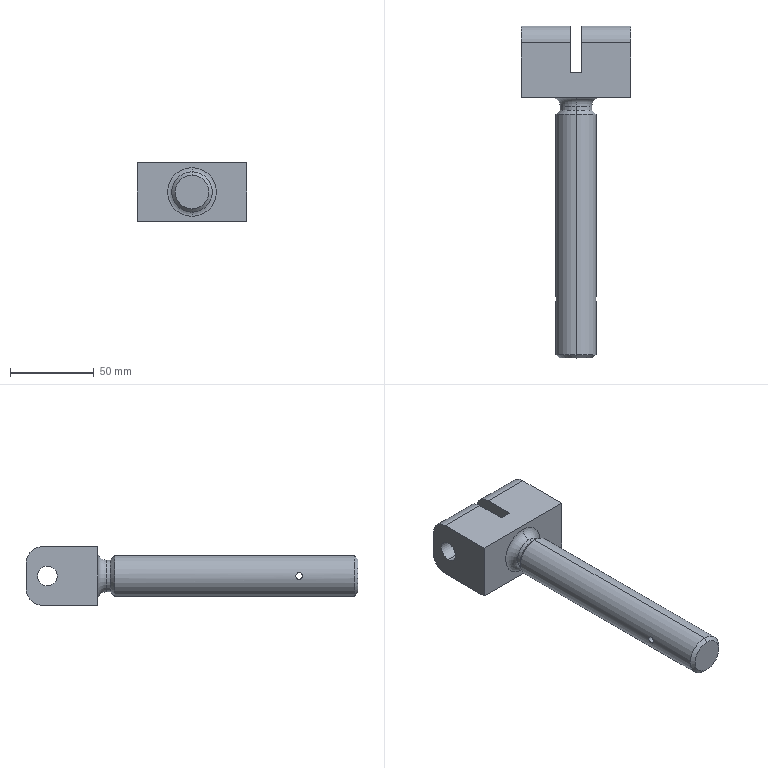Part | SolidWorks | features MBimport 1 | 1 solid | 31 faces | box 65.4 x 197.7 x 35 mm | volume 150563 mm3 | cylinder 14 | plane 11 | cone 4 | torus 2 | commonest cylinder face diameters 11.775 x4 20 x4 4 x2 19 x2 24 x2
STEP:
#1=CARTESIAN_POINT('',(20.868,-128.108,12.8));
#2=VERTEX_POINT('',#1);
#3=CARTESIAN_POINT('',(44.532,-128.108,12.8));
#4=VERTEX_POINT('',#3);
#5=CARTESIAN_POINT('',(0.,-128.108,12.8));
#6=DIRECTION('',(1.,0.,0.));
#7=VECTOR('',#6,1000.);
#8=LINE('',#5,#7);
#9=EDGE_CURVE('',#2,#4,#8,.T.);
#10=ORIENTED_EDGE('',*,*,#9,.F.);
#11=CARTESIAN_POINT('',(20.868,-128.108,8.8));
#12=VERTEX_POINT('',#11);
#13=CARTESIAN_POINT('',(20.868,-128.108,12.8));
#14=CARTESIAN_POINT('',(20.868,-127.984,12.8));
#15=CARTESIAN_POINT('',(20.866,-127.857,12.789));
#16=CARTESIAN_POINT('',(20.86,-127.664,12.751));
#17=CARTESIAN_POINT('',(20.857,-127.599,12.736));
#18=CARTESIAN_POINT('',(20.852,-127.503,12.707));
#19=CARTESIAN_POINT('',(20.85,-127.454,12.691));
#20=CARTESIAN_POINT('',(20.847,-127.398,12.67));
#21=CARTESIAN_POINT('',(20.845,-127.37,12.659));
#22=CARTESIAN_POINT('',(20.844,-127.358,12.654));
#23=CARTESIAN_POINT('',(20.844,-127.35,12.651));
#24=CARTESIAN_POINT('',(20.843,-127.345,12.649));
#25=CARTESIAN_POINT('',(20.838,-127.261,12.614));
#26=CARTESIAN_POINT('',(20.83,-127.162,12.567));
#27=CARTESIAN_POINT('',(20.81,-126.94,12.429));
#28=CARTESIAN_POINT('',(20.798,-126.816,12.337));
#29=CARTESIAN_POINT('',(20.769,-126.573,12.094));
#30=CARTESIAN_POINT('',(20.757,-126.482,11.972));
#31=CARTESIAN_POINT('',(20.742,-126.378,11.806));
#32=CARTESIAN_POINT('',(20.738,-126.349,11.753));
#33=CARTESIAN_POINT('',(20.732,-126.311,11.679));
#34=CARTESIAN_POINT('',(20.731,-126.3,11.656));
#35=CARTESIAN_POINT('',(20.728,-126.284,11.622));
#36=CARTESIAN_POINT('',(20.727,-126.277,11.605));
#37=CARTESIAN_POINT('',(20.726,-126.269,11.586));
#38=CARTESIAN_POINT('',(20.725,-126.265,11.578));
#39=CARTESIAN_POINT('',(20.725,-126.263,11.573));
#40=CARTESIAN_POINT('',(20.725,-126.263,11.572));
#41=CARTESIAN_POINT('',(20.708,-126.155,11.313));
#42=CARTESIAN_POINT('',(20.7,-126.108,11.049));
#43=CARTESIAN_POINT('',(20.7,-126.108,10.677));
#44=CARTESIAN_POINT('',(20.702,-126.119,10.55));
#45=CARTESIAN_POINT('',(20.708,-126.156,10.357));
#46=CARTESIAN_POINT('',(20.711,-126.172,10.292));
#47=CARTESIAN_POINT('',(20.715,-126.201,10.195));
#48=CARTESIAN_POINT('',(20.718,-126.217,10.147));
#49=CARTESIAN_POINT('',(20.721,-126.238,10.091));
#50=CARTESIAN_POINT('',(20.723,-126.249,10.063));
#51=CARTESIAN_POINT('',(20.723,-126.253,10.051));
#52=CARTESIAN_POINT('',(20.724,-126.257,10.043));
#53=CARTESIAN_POINT('',(20.724,-126.259,10.037));
#54=CARTESIAN_POINT('',(20.73,-126.294,9.952));
#55=CARTESIAN_POINT('',(20.737,-126.342,9.852));
#56=CARTESIAN_POINT('',(20.757,-126.481,9.63));
#57=CARTESIAN_POINT('',(20.769,-126.57,9.51));
#58=CARTESIAN_POINT('',(20.798,-126.815,9.264));
#59=CARTESIAN_POINT('',(20.81,-126.938,9.173));
#60=CARTESIAN_POINT('',(20.825,-127.104,9.069));
#61=CARTESIAN_POINT('',(20.83,-127.157,9.04));
#62=CARTESIAN_POINT('',(20.835,-127.23,9.003));
#63=CARTESIAN_POINT('',(20.837,-127.253,8.992));
#64=CARTESIAN_POINT('',(20.839,-127.287,8.976));
#65=CARTESIAN_POINT('',(20.841,-127.303,8.969));
#66=CARTESIAN_POINT('',(20.842,-127.322,8.961));
#67=CARTESIAN_POINT('',(20.842,-127.329,8.958));
#68=CARTESIAN_POINT('',(20.843,-127.335,8.956));
#69=CARTESIAN_POINT('',(20.843,-127.336,8.955));
#70=CARTESIAN_POINT('',(20.86,-127.596,8.847));
#71=CARTESIAN_POINT('',(20.868,-127.86,8.8));
#72=CARTESIAN_POINT('',(20.868,-128.108,8.8));
#73=B_SPLINE_CURVE_WITH_KNOTS('',3,(#13,#14,#15,#16,#17,#18,#19,#20,#21,#22,#23,#24,#25,#26,#27,#28,#29,#30,#31,#32,#33,#34,#35,#36,#37,#38,#39,#40,#41,#42,#43,#44,#45,#46,#47,#48,#49,#50,#51,#52,#53,#54,#55,#56,#57,#58,#59,#60,#61,#62,#63,#64,#65,#66,#67,#68,#69,#70,#71,#72),.UNSPECIFIED.,.F.,.F.,(4,2,2,1,1,1,2,2,2,2,2,2,2,1,1,2,2,2,2,2,1,1,1,2,2,2,2,2,2,2,1,1,2,2,4),(0.,0.0625,0.09375,0.1094,0.1172,0.1211,0.123,0.125,0.1875,0.25,0.3125,0.3438,0.3594,0.3672,0.3711,0.373,0.375,0.5,0.5625,0.5938,0.6094,0.6172,0.6211,0.623,0.625,0.6875,0.75,0.8125,0.8438,0.8594,0.8672,0.8711,0.873,0.875,1.),.UNSPECIFIED.);
#74=EDGE_CURVE('',#2,#12,#73,.T.);
#75=ORIENTED_EDGE('',*,*,#74,.T.);
#76=CARTESIAN_POINT('',(44.532,-128.108,8.8));
#77=VERTEX_POINT('',#76);
#78=CARTESIAN_POINT('',(0.,-128.108,8.8));
#79=DIRECTION('',(1.,0.,0.));
#80=VECTOR('',#79,1000.);
#81=LINE('',#78,#80);
#82=EDGE_CURVE('',#12,#77,#81,.T.);
#83=ORIENTED_EDGE('',*,*,#82,.T.);
#84=CARTESIAN_POINT('',(44.532,-128.108,8.8));
#85=CARTESIAN_POINT('',(44.532,-127.984,8.8));
#86=CARTESIAN_POINT('',(44.534,-127.856,8.812));
#87=CARTESIAN_POINT('',(44.54,-127.663,8.849));
#88=CARTESIAN_POINT('',(44.543,-127.599,8.865));
#89=CARTESIAN_POINT('',(44.548,-127.502,8.894));
#90=CARTESIAN_POINT('',(44.55,-127.453,8.91));
#91=CARTESIAN_POINT('',(44.553,-127.397,8.93));
#92=CARTESIAN_POINT('',(44.555,-127.369,8.941));
#93=CARTESIAN_POINT('',(44.556,-127.357,8.946));
#94=CARTESIAN_POINT('',(44.556,-127.349,8.95));
#95=CARTESIAN_POINT('',(44.557,-127.344,8.952));
#96=CARTESIAN_POINT('',(44.562,-127.26,8.987));
#97=CARTESIAN_POINT('',(44.57,-127.161,9.034));
#98=CARTESIAN_POINT('',(44.585,-126.994,9.137));
#99=CARTESIAN_POINT('',(44.59,-126.936,9.178));
#100=CARTESIAN_POINT('',(44.602,-126.816,9.271));
#101=CARTESIAN_POINT('',(44.609,-126.754,9.326));
#102=CARTESIAN_POINT('',(44.631,-126.572,9.507));
#103=CARTESIAN_POINT('',(44.643,-126.481,9.629));
#104=CARTESIAN_POINT('',(44.658,-126.377,9.795));
#105=CARTESIAN_POINT('',(44.662,-126.348,9.848));
#106=CARTESIAN_POINT('',(44.668,-126.311,9.922));
#107=CARTESIAN_POINT('',(44.669,-126.299,9.946));
#108=CARTESIAN_POINT('',(44.672,-126.284,9.98));
#109=CARTESIAN_POINT('',(44.673,-126.276,9.997));
#110=CARTESIAN_POINT('',(44.674,-126.268,10.015));
#111=CARTESIAN_POINT('',(44.675,-126.265,10.023));
#112=CARTESIAN_POINT('',(44.675,-126.263,10.029));
#113=CARTESIAN_POINT('',(44.675,-126.262,10.03));
#114=CARTESIAN_POINT('',(44.692,-126.155,10.289));
#115=CARTESIAN_POINT('',(44.7,-126.108,10.551));
#116=CARTESIAN_POINT('',(44.7,-126.108,10.923));
#117=CARTESIAN_POINT('',(44.698,-126.119,11.051));
#118=CARTESIAN_POINT('',(44.692,-126.156,11.244));
#119=CARTESIAN_POINT('',(44.689,-126.172,11.308));
#120=CARTESIAN_POINT('',(44.685,-126.201,11.405));
#121=CARTESIAN_POINT('',(44.682,-126.217,11.453));
#122=CARTESIAN_POINT('',(44.679,-126.238,11.51));
#123=CARTESIAN_POINT('',(44.677,-126.249,11.538));
#124=CARTESIAN_POINT('',(44.677,-126.253,11.55));
#125=CARTESIAN_POINT('',(44.676,-126.257,11.558));
#126=CARTESIAN_POINT('',(44.676,-126.259,11.563));
#127=CARTESIAN_POINT('',(44.67,-126.294,11.649));
#128=CARTESIAN_POINT('',(44.663,-126.342,11.749));
#129=CARTESIAN_POINT('',(44.643,-126.481,11.971));
#130=CARTESIAN_POINT('',(44.631,-126.571,12.092));
#131=CARTESIAN_POINT('',(44.602,-126.816,12.337));
#132=CARTESIAN_POINT('',(44.59,-126.939,12.428));
#133=CARTESIAN_POINT('',(44.575,-127.106,12.532));
#134=CARTESIAN_POINT('',(44.57,-127.158,12.561));
#135=CARTESIAN_POINT('',(44.565,-127.232,12.598));
#136=CARTESIAN_POINT('',(44.563,-127.255,12.609));
#137=CARTESIAN_POINT('',(44.56,-127.289,12.625));
#138=CARTESIAN_POINT('',(44.559,-127.305,12.632));
#139=CARTESIAN_POINT('',(44.558,-127.324,12.64));
#140=CARTESIAN_POINT('',(44.558,-127.332,12.643));
#141=CARTESIAN_POINT('',(44.557,-127.337,12.646));
#142=CARTESIAN_POINT('',(44.557,-127.338,12.646));
#143=CARTESIAN_POINT('',(44.54,-127.597,12.754));
#144=CARTESIAN_POINT('',(44.532,-127.86,12.8));
#145=CARTESIAN_POINT('',(44.532,-128.108,12.8));
#146=B_SPLINE_CURVE_WITH_KNOTS('',3,(#84,#85,#86,#87,#88,#89,#90,#91,#92,#93,#94,#95,#96,#97,#98,#99,#100,#101,#102,#103,#104,#105,#106,#107,#108,#109,#110,#111,#112,#113,#114,#115,#116,#117,#118,#119,#120,#121,#122,#123,#124,#125,#126,#127,#128,#129,#130,#131,#132,#133,#134,#135,#136,#137,#138,#139,#140,#141,#142,#143,#144,#145),.UNSPECIFIED.,.F.,.F.,(4,2,2,1,1,1,2,2,2,2,2,2,2,2,1,1,2,2,2,2,2,1,1,1,2,2,2,2,2,2,2,1,1,2,2,4),(0.,0.0625,0.09375,0.1094,0.1172,0.1211,0.123,0.125,0.1875,0.2188,0.25,0.3125,0.3438,0.3594,0.3672,0.3711,0.373,0.375,0.5,0.5625,0.5938,0.6094,0.6172,0.6211,0.623,0.625,0.6875,0.75,0.8125,0.8437,0.8594,0.8672,0.8711,0.873,0.875,1.),.UNSPECIFIED.);
#147=EDGE_CURVE('',#77,#4,#146,.T.);
#148=ORIENTED_EDGE('',*,*,#147,.T.);
#149=EDGE_LOOP('',(#10,#75,#83,#148));
#150=FACE_OUTER_BOUND('',#149,.T.);
#151=CARTESIAN_POINT('',(0.,-128.108,10.8));
#152=DIRECTION('',(1.,0.,0.));
#153=DIRECTION('',(0.,0.,-1.));
#154=AXIS2_PLACEMENT_3D('',#151,#152,#153);
#155=CYLINDRICAL_SURFACE('',#154,2.);
#156=ADVANCED_FACE('',(#150),#155,.F.);
#157=CARTESIAN_POINT('',(36.2,21.892,16.688));
#158=VERTEX_POINT('',#157);
#159=CARTESIAN_POINT('',(36.2,21.892,4.912));
#160=VERTEX_POINT('',#159);
#161=CARTESIAN_POINT('',(36.2,21.892,10.8));
#162=DIRECTION('',(-1.,0.,0.));
#163=DIRECTION('',(0.,0.,1.));
#164=AXIS2_PLACEMENT_3D('',#161,#162,#163);
#165=CIRCLE('',#164,5.888);
#166=EDGE_CURVE('',#158,#160,#165,.T.);
#167=ORIENTED_EDGE('',*,*,#166,.F.);
#168=CARTESIAN_POINT('',(36.2,21.892,10.8));
#169=DIRECTION('',(-1.,0.,0.));
#170=DIRECTION('',(0.,0.,1.));
#171=AXIS2_PLACEMENT_3D('',#168,#169,#170);
#172=CIRCLE('',#171,5.888);
#173=EDGE_CURVE('',#160,#158,#172,.T.);
#174=ORIENTED_EDGE('',*,*,#173,.F.);
#175=EDGE_LOOP('',(#167,#174));
#176=FACE_BOUND('',#175,.T.);
#177=CARTESIAN_POINT('',(36.2,34.592,3.3));
#178=VERTEX_POINT('',#177);
#179=CARTESIAN_POINT('',(36.2,24.592,-6.7));
#180=VERTEX_POINT('',#179);
#181=CARTESIAN_POINT('',(36.2,24.592,3.3));
#182=DIRECTION('',(-1.,0.,0.));
#183=DIRECTION('',(0.,0.,1.));
#184=AXIS2_PLACEMENT_3D('',#181,#182,#183);
#185=CIRCLE('',#184,10.);
#186=EDGE_CURVE('',#178,#180,#185,.T.);
#187=ORIENTED_EDGE('',*,*,#186,.T.);
#188=CARTESIAN_POINT('',(36.2,6.592,-6.7));
#189=VERTEX_POINT('',#188);
#190=CARTESIAN_POINT('',(36.2,24.592,-6.7));
#191=DIRECTION('',(0.,-1.,0.));
#192=VECTOR('',#191,1000.);
#193=LINE('',#190,#192);
#194=EDGE_CURVE('',#180,#189,#193,.T.);
#195=ORIENTED_EDGE('',*,*,#194,.T.);
#196=CARTESIAN_POINT('',(36.2,6.592,28.3));
#197=VERTEX_POINT('',#196);
#198=CARTESIAN_POINT('',(36.2,6.592,335.997));
#199=DIRECTION('',(0.,0.,-1.));
#200=VECTOR('',#199,1000.);
#201=LINE('',#198,#200);
#202=EDGE_CURVE('',#197,#189,#201,.T.);
#203=ORIENTED_EDGE('',*,*,#202,.F.);
#204=CARTESIAN_POINT('',(36.2,24.592,28.3));
#205=VERTEX_POINT('',#204);
#206=CARTESIAN_POINT('',(36.2,24.592,28.3));
#207=DIRECTION('',(0.,1.,0.));
#208=VECTOR('',#207,1000.);
#209=LINE('',#206,#208);
#210=EDGE_CURVE('',#197,#205,#209,.T.);
#211=ORIENTED_EDGE('',*,*,#210,.T.);
#212=CARTESIAN_POINT('',(36.2,34.592,18.3));
#213=VERTEX_POINT('',#212);
#214=CARTESIAN_POINT('',(36.2,24.592,18.3));
#215=DIRECTION('',(-1.,0.,0.));
#216=DIRECTION('',(0.,0.,1.));
#217=AXIS2_PLACEMENT_3D('',#214,#215,#216);
#218=CIRCLE('',#217,10.);
#219=EDGE_CURVE('',#205,#213,#218,.T.);
#220=ORIENTED_EDGE('',*,*,#219,.T.);
#221=CARTESIAN_POINT('',(36.2,34.592,335.997));
#222=DIRECTION('',(0.,0.,-1.));
#223=VECTOR('',#222,1000.);
#224=LINE('',#221,#223);
#225=EDGE_CURVE('',#213,#178,#224,.T.);
#226=ORIENTED_EDGE('',*,*,#225,.T.);
#227=EDGE_LOOP('',(#187,#195,#203,#211,#220,#226));
#228=FACE_OUTER_BOUND('',#227,.T.);
#229=CARTESIAN_POINT('',(36.2,6.592,335.997));
#230=DIRECTION('',(-1.,0.,0.));
#231=DIRECTION('',(0.,0.,1.));
#232=AXIS2_PLACEMENT_3D('',#229,#230,#231);
#233=PLANE('',#232);
#234=ADVANCED_FACE('',(#176,#228),#233,.T.);
#235=CARTESIAN_POINT('',(29.2,21.892,16.688));
#236=VERTEX_POINT('',#235);
#237=CARTESIAN_POINT('',(29.2,21.892,4.912));
#238=VERTEX_POINT('',#237);
#239=CARTESIAN_POINT('',(29.2,21.892,10.8));
#240=DIRECTION('',(1.,0.,0.));
#241=DIRECTION('',(0.,1.,0.));
#242=AXIS2_PLACEMENT_3D('',#239,#240,#241);
#243=CIRCLE('',#242,5.888);
#244=EDGE_CURVE('',#236,#238,#243,.T.);
#245=ORIENTED_EDGE('',*,*,#244,.F.);
#246=CARTESIAN_POINT('',(29.2,21.892,10.8));
#247=DIRECTION('',(1.,0.,0.));
#248=DIRECTION('',(0.,1.,0.));
#249=AXIS2_PLACEMENT_3D('',#246,#247,#248);
#250=CIRCLE('',#249,5.888);
#251=EDGE_CURVE('',#238,#236,#250,.T.);
#252=ORIENTED_EDGE('',*,*,#251,.F.);
#253=EDGE_LOOP('',(#245,#252));
#254=FACE_BOUND('',#253,.T.);
#255=CARTESIAN_POINT('',(29.2,6.592,28.3));
#256=VERTEX_POINT('',#255);
#257=CARTESIAN_POINT('',(29.2,6.592,-6.7));
#258=VERTEX_POINT('',#257);
#259=CARTESIAN_POINT('',(29.2,6.592,335.997));
#260=DIRECTION('',(0.,0.,-1.));
#261=VECTOR('',#260,1000.);
#262=LINE('',#259,#261);
#263=EDGE_CURVE('',#256,#258,#262,.T.);
#264=ORIENTED_EDGE('',*,*,#263,.T.);
#265=CARTESIAN_POINT('',(29.2,24.592,-6.7));
#266=VERTEX_POINT('',#265);
#267=CARTESIAN_POINT('',(29.2,24.592,-6.7));
#268=DIRECTION('',(0.,1.,0.));
#269=VECTOR('',#268,1000.);
#270=LINE('',#267,#269);
#271=EDGE_CURVE('',#258,#266,#270,.T.);
#272=ORIENTED_EDGE('',*,*,#271,.T.);
#273=CARTESIAN_POINT('',(29.2,34.592,3.3));
#274=VERTEX_POINT('',#273);
#275=CARTESIAN_POINT('',(29.2,24.592,3.3));
#276=DIRECTION('',(1.,0.,0.));
#277=DIRECTION('',(0.,1.,0.));
#278=AXIS2_PLACEMENT_3D('',#275,#276,#277);
#279=CIRCLE('',#278,10.);
#280=EDGE_CURVE('',#266,#274,#279,.T.);
#281=ORIENTED_EDGE('',*,*,#280,.T.);
#282=CARTESIAN_POINT('',(29.2,34.592,18.3));
#283=VERTEX_POINT('',#282);
#284=CARTESIAN_POINT('',(29.2,34.592,335.997));
#285=DIRECTION('',(0.,0.,-1.));
#286=VECTOR('',#285,1000.);
#287=LINE('',#284,#286);
#288=EDGE_CURVE('',#283,#274,#287,.T.);
#289=ORIENTED_EDGE('',*,*,#288,.F.);
#290=CARTESIAN_POINT('',(29.2,24.592,28.3));
#291=VERTEX_POINT('',#290);
#292=CARTESIAN_POINT('',(29.2,24.592,18.3));
#293=DIRECTION('',(1.,0.,0.));
#294=DIRECTION('',(0.,1.,0.));
#295=AXIS2_PLACEMENT_3D('',#292,#293,#294);
#296=CIRCLE('',#295,10.);
#297=EDGE_CURVE('',#283,#291,#296,.T.);
#298=ORIENTED_EDGE('',*,*,#297,.T.);
#299=CARTESIAN_POINT('',(29.2,24.592,28.3));
#300=DIRECTION('',(0.,-1.,0.));
#301=VECTOR('',#300,1000.);
#302=LINE('',#299,#301);
#303=EDGE_CURVE('',#291,#256,#302,.T.);
#304=ORIENTED_EDGE('',*,*,#303,.T.);
#305=EDGE_LOOP('',(#264,#272,#281,#289,#298,#304));
#306=FACE_OUTER_BOUND('',#305,.T.);
#307=CARTESIAN_POINT('',(29.2,34.592,335.997));
#308=DIRECTION('',(1.,0.,0.));
#309=DIRECTION('',(0.,1.,0.));
#310=AXIS2_PLACEMENT_3D('',#307,#308,#309);
#311=PLANE('',#310);
#312=ADVANCED_FACE('',(#254,#306),#311,.T.);
#313=ORIENTED_EDGE('',*,*,#202,.T.);
#314=CARTESIAN_POINT('',(65.4,6.592,-6.7));
#315=DIRECTION('',(-1.,0.,0.));
#316=VECTOR('',#315,1000.);
#317=LINE('',#314,#316);
#318=EDGE_CURVE('',#189,#258,#317,.T.);
#319=ORIENTED_EDGE('',*,*,#318,.T.);
#320=ORIENTED_EDGE('',*,*,#263,.F.);
#321=CARTESIAN_POINT('',(65.4,6.592,28.3));
#322=DIRECTION('',(1.,0.,0.));
#323=VECTOR('',#322,1000.);
#324=LINE('',#321,#323);
#325=EDGE_CURVE('',#256,#197,#324,.T.);
#326=ORIENTED_EDGE('',*,*,#325,.T.);
#327=EDGE_LOOP('',(#313,#319,#320,#326));
#328=FACE_OUTER_BOUND('',#327,.T.);
#329=CARTESIAN_POINT('',(29.2,6.592,335.997));
#330=DIRECTION('',(0.,1.,0.));
#331=DIRECTION('',(1.,0.,0.));
#332=AXIS2_PLACEMENT_3D('',#329,#330,#331);
#333=PLANE('',#332);
#334=ADVANCED_FACE('',(#328),#333,.T.);
#335=CARTESIAN_POINT('',(32.7,-163.108,0.8001));
#336=VERTEX_POINT('',#335);
#337=CARTESIAN_POINT('',(32.7,-161.108,-1.2));
#338=VERTEX_POINT('',#337);
#339=CARTESIAN_POINT('',(32.7,-161.108,-1.2));
#340=DIRECTION('',(0.,0.7071,-0.7071));
#341=VECTOR('',#340,1000.);
#342=LINE('',#339,#341);
#343=EDGE_CURVE('',#336,#338,#342,.T.);
#344=ORIENTED_EDGE('',*,*,#343,.F.);
#345=CARTESIAN_POINT('',(32.7,-163.108,20.8));
#346=VERTEX_POINT('',#345);
#347=CARTESIAN_POINT('',(32.7,-163.108,10.8));
#348=DIRECTION('',(0.,-1.,0.));
#349=DIRECTION('',(0.,0.,-1.));
#350=AXIS2_PLACEMENT_3D('',#347,#348,#349);
#351=CIRCLE('',#350,10.);
#352=EDGE_CURVE('',#346,#336,#351,.T.);
#353=ORIENTED_EDGE('',*,*,#352,.F.);
#354=CARTESIAN_POINT('',(32.7,-161.108,22.8));
#355=VERTEX_POINT('',#354);
#356=CARTESIAN_POINT('',(32.7,-161.108,22.8));
#357=DIRECTION('',(0.,0.7071,0.7071));
#358=VECTOR('',#357,1000.);
#359=LINE('',#356,#358);
#360=EDGE_CURVE('',#346,#355,#359,.T.);
#361=ORIENTED_EDGE('',*,*,#360,.T.);
#362=CARTESIAN_POINT('',(32.7,-161.108,10.8));
#363=DIRECTION('',(0.,1.,0.));
#364=DIRECTION('',(0.,0.,-1.));
#365=AXIS2_PLACEMENT_3D('',#362,#363,#364);
#366=CIRCLE('',#365,12.);
#367=EDGE_CURVE('',#338,#355,#366,.T.);
#368=ORIENTED_EDGE('',*,*,#367,.F.);
#369=EDGE_LOOP('',(#344,#353,#361,#368));
#370=FACE_OUTER_BOUND('',#369,.T.);
#371=CARTESIAN_POINT('',(32.7,-161.108,10.8));
#372=DIRECTION('',(0.,1.,0.));
#373=DIRECTION('',(0.,0.,1.));
#374=AXIS2_PLACEMENT_3D('',#371,#372,#373);
#375=CONICAL_SURFACE('',#374,12.,0.7854);
#376=ADVANCED_FACE('',(#370),#375,.T.);
#377=ORIENTED_EDGE('',*,*,#352,.T.);
#378=CARTESIAN_POINT('',(32.7,-163.108,10.8));
#379=DIRECTION('',(0.,-1.,0.));
#380=DIRECTION('',(0.,0.,-1.));
#381=AXIS2_PLACEMENT_3D('',#378,#379,#380);
#382=CIRCLE('',#381,10.);
#383=EDGE_CURVE('',#336,#346,#382,.T.);
#384=ORIENTED_EDGE('',*,*,#383,.T.);
#385=EDGE_LOOP('',(#377,#384));
#386=FACE_OUTER_BOUND('',#385,.T.);
#387=CARTESIAN_POINT('',(32.7,-163.108,0.));
#388=DIRECTION('',(0.,-1.,0.));
#389=DIRECTION('',(0.,0.,-1.));
#390=AXIS2_PLACEMENT_3D('',#387,#388,#389);
#391=PLANE('',#390);
#392=ADVANCED_FACE('',(#386),#391,.T.);
#393=CARTESIAN_POINT('',(20.868,-128.108,8.8));
#394=CARTESIAN_POINT('',(20.868,-128.232,8.8));
#395=CARTESIAN_POINT('',(20.866,-128.359,8.812));
#396=CARTESIAN_POINT('',(20.86,-128.552,8.849));
#397=CARTESIAN_POINT('',(20.857,-128.617,8.865));
#398=CARTESIAN_POINT('',(20.852,-128.714,8.894));
#399=CARTESIAN_POINT('',(20.85,-128.762,8.91));
#400=CARTESIAN_POINT('',(20.847,-128.818,8.93));
#401=CARTESIAN_POINT('',(20.845,-128.846,8.941));
#402=CARTESIAN_POINT('',(20.844,-128.858,8.946));
#403=CARTESIAN_POINT('',(20.844,-128.866,8.95));
#404=CARTESIAN_POINT('',(20.843,-128.872,8.952));
#405=CARTESIAN_POINT('',(20.838,-128.956,8.987));
#406=CARTESIAN_POINT('',(20.83,-129.055,9.034));
#407=CARTESIAN_POINT('',(20.815,-129.221,9.137));
#408=CARTESIAN_POINT('',(20.81,-129.28,9.178));
#409=CARTESIAN_POINT('',(20.798,-129.399,9.271));
#410=CARTESIAN_POINT('',(20.791,-129.462,9.326));
#411=CARTESIAN_POINT('',(20.769,-129.643,9.507));
#412=CARTESIAN_POINT('',(20.757,-129.734,9.629));
#413=CARTESIAN_POINT('',(20.742,-129.838,9.795));
#414=CARTESIAN_POINT('',(20.738,-129.868,9.848));
#415=CARTESIAN_POINT('',(20.732,-129.905,9.922));
#416=CARTESIAN_POINT('',(20.731,-129.916,9.946));
#417=CARTESIAN_POINT('',(20.728,-129.932,9.98));
#418=CARTESIAN_POINT('',(20.727,-129.939,9.997));
#419=CARTESIAN_POINT('',(20.726,-129.947,10.015));
#420=CARTESIAN_POINT('',(20.725,-129.951,10.023));
#421=CARTESIAN_POINT('',(20.725,-129.953,10.029));
#422=CARTESIAN_POINT('',(20.725,-129.953,10.03));
#423=CARTESIAN_POINT('',(20.708,-130.061,10.289));
#424=CARTESIAN_POINT('',(20.7,-130.108,10.551));
#425=CARTESIAN_POINT('',(20.7,-130.108,10.923));
#426=CARTESIAN_POINT('',(20.702,-130.096,11.051));
#427=CARTESIAN_POINT('',(20.708,-130.059,11.244));
#428=CARTESIAN_POINT('',(20.711,-130.043,11.308));
#429=CARTESIAN_POINT('',(20.715,-130.014,11.405));
#430=CARTESIAN_POINT('',(20.718,-129.999,11.453));
#431=CARTESIAN_POINT('',(20.721,-129.978,11.51));
#432=CARTESIAN_POINT('',(20.723,-129.967,11.538));
#433=CARTESIAN_POINT('',(20.723,-129.962,11.55));
#434=CARTESIAN_POINT('',(20.724,-129.959,11.558));
#435=CARTESIAN_POINT('',(20.724,-129.957,11.563));
#436=CARTESIAN_POINT('',(20.73,-129.921,11.649));
#437=CARTESIAN_POINT('',(20.737,-129.873,11.749));
#438=CARTESIAN_POINT('',(20.757,-129.735,11.971));
#439=CARTESIAN_POINT('',(20.769,-129.645,12.092));
#440=CARTESIAN_POINT('',(20.798,-129.399,12.337));
#441=CARTESIAN_POINT('',(20.81,-129.276,12.428));
#442=CARTESIAN_POINT('',(20.825,-129.11,12.532));
#443=CARTESIAN_POINT('',(20.83,-129.057,12.561));
#444=CARTESIAN_POINT('',(20.835,-128.984,12.598));
#445=CARTESIAN_POINT('',(20.837,-128.96,12.609));
#446=CARTESIAN_POINT('',(20.84,-128.927,12.625));
#447=CARTESIAN_POINT('',(20.841,-128.91,12.632));
#448=CARTESIAN_POINT('',(20.842,-128.892,12.64));
#449=CARTESIAN_POINT('',(20.842,-128.884,12.643));
#450=CARTESIAN_POINT('',(20.843,-128.879,12.646));
#451=CARTESIAN_POINT('',(20.843,-128.878,12.646));
#452=CARTESIAN_POINT('',(20.86,-128.618,12.754));
#453=CARTESIAN_POINT('',(20.868,-128.355,12.8));
#454=CARTESIAN_POINT('',(20.868,-128.108,12.8));
#455=B_SPLINE_CURVE_WITH_KNOTS('',3,(#393,#394,#395,#396,#397,#398,#399,#400,#401,#402,#403,#404,#405,#406,#407,#408,#409,#410,#411,#412,#413,#414,#415,#416,#417,#418,#419,#420,#421,#422,#423,#424,#425,#426,#427,#428,#429,#430,#431,#432,#433,#434,#435,#436,#437,#438,#439,#440,#441,#442,#443,#444,#445,#446,#447,#448,#449,#450,#451,#452,#453,#454),.UNSPECIFIED.,.F.,.F.,(4,2,2,1,1,1,2,2,2,2,2,2,2,2,1,1,2,2,2,2,2,1,1,1,2,2,2,2,2,2,2,1,1,2,2,4),(0.,0.0625,0.09375,0.1094,0.1172,0.1211,0.123,0.125,0.1875,0.2187,0.25,0.3125,0.3437,0.3594,0.3672,0.3711,0.373,0.375,0.5,0.5625,0.5937,0.6094,0.6172,0.6211,0.623,0.625,0.6875,0.75,0.8125,0.8437,0.8594,0.8672,0.8711,0.873,0.875,1.),.UNSPECIFIED.);
#456=EDGE_CURVE('',#12,#2,#455,.T.);
#457=ORIENTED_EDGE('',*,*,#456,.F.);
#458=ORIENTED_EDGE('',*,*,#74,.F.);
#459=EDGE_LOOP('',(#457,#458));
#460=FACE_BOUND('',#459,.T.);
#461=CARTESIAN_POINT('',(32.7,-18.108,-1.2));
#462=VERTEX_POINT('',#461);
#463=CARTESIAN_POINT('',(32.7,34.592,-1.2));
#464=DIRECTION('',(0.,1.,0.));
#465=VECTOR('',#464,1000.);
#466=LINE('',#463,#465);
#467=EDGE_CURVE('',#338,#462,#466,.T.);
#468=ORIENTED_EDGE('',*,*,#467,.F.);
#469=ORIENTED_EDGE('',*,*,#367,.T.);
#470=CARTESIAN_POINT('',(32.7,-18.108,22.8));
#471=VERTEX_POINT('',#470);
#472=CARTESIAN_POINT('',(32.7,34.592,22.8));
#473=DIRECTION('',(0.,1.,0.));
#474=VECTOR('',#473,1000.);
#475=LINE('',#472,#474);
#476=EDGE_CURVE('',#355,#471,#475,.T.);
#477=ORIENTED_EDGE('',*,*,#476,.T.);
#478=CARTESIAN_POINT('',(32.7,-18.108,10.8));
#479=DIRECTION('',(0.,1.,0.));
#480=DIRECTION('',(0.,0.,1.));
#481=AXIS2_PLACEMENT_3D('',#478,#479,#480);
#482=CIRCLE('',#481,12.);
#483=EDGE_CURVE('',#462,#471,#482,.T.);
#484=ORIENTED_EDGE('',*,*,#483,.F.);
#485=EDGE_LOOP('',(#468,#469,#477,#484));
#486=FACE_OUTER_BOUND('',#485,.T.);
#487=CARTESIAN_POINT('',(32.7,34.592,10.8));
#488=DIRECTION('',(0.,1.,0.));
#489=DIRECTION('',(0.,0.,1.));
#490=AXIS2_PLACEMENT_3D('',#487,#488,#489);
#491=CYLINDRICAL_SURFACE('',#490,12.);
#492=ADVANCED_FACE('',(#460,#486),#491,.T.);
#493=CARTESIAN_POINT('',(32.7,-15.608,20.3));
#494=VERTEX_POINT('',#493);
#495=CARTESIAN_POINT('',(32.7,-18.108,22.8));
#496=DIRECTION('',(0.,-0.7071,0.7071));
#497=VECTOR('',#496,1000.);
#498=LINE('',#495,#497);
#499=EDGE_CURVE('',#494,#471,#498,.T.);
#500=ORIENTED_EDGE('',*,*,#499,.F.);
#501=CARTESIAN_POINT('',(32.7,-15.608,1.3));
#502=VERTEX_POINT('',#501);
#503=CARTESIAN_POINT('',(32.7,-15.608,10.8));
#504=DIRECTION('',(0.,1.,0.));
#505=DIRECTION('',(0.,0.,1.));
#506=AXIS2_PLACEMENT_3D('',#503,#504,#505);
#507=CIRCLE('',#506,9.5);
#508=EDGE_CURVE('',#502,#494,#507,.T.);
#509=ORIENTED_EDGE('',*,*,#508,.F.);
#510=CARTESIAN_POINT('',(32.7,-18.108,-1.2));
#511=DIRECTION('',(0.,-0.7071,-0.7071));
#512=VECTOR('',#511,1000.);
#513=LINE('',#510,#512);
#514=EDGE_CURVE('',#502,#462,#513,.T.);
#515=ORIENTED_EDGE('',*,*,#514,.T.);
#516=ORIENTED_EDGE('',*,*,#483,.T.);
#517=EDGE_LOOP('',(#500,#509,#515,#516));
#518=FACE_OUTER_BOUND('',#517,.T.);
#519=CARTESIAN_POINT('',(32.7,-18.108,10.8));
#520=DIRECTION('',(0.,-1.,0.));
#521=DIRECTION('',(0.,0.,-1.));
#522=AXIS2_PLACEMENT_3D('',#519,#520,#521);
#523=CONICAL_SURFACE('',#522,12.,0.7854);
#524=ADVANCED_FACE('',(#518),#523,.T.);
#525=CARTESIAN_POINT('',(32.7,-13.108,1.3));
#526=VERTEX_POINT('',#525);
#527=CARTESIAN_POINT('',(32.7,34.592,1.3));
#528=DIRECTION('',(0.,1.,0.));
#529=VECTOR('',#528,1000.);
#530=LINE('',#527,#529);
#531=EDGE_CURVE('',#502,#526,#530,.T.);
#532=ORIENTED_EDGE('',*,*,#531,.F.);
#533=ORIENTED_EDGE('',*,*,#508,.T.);
#534=CARTESIAN_POINT('',(32.7,-13.108,20.3));
#535=VERTEX_POINT('',#534);
#536=CARTESIAN_POINT('',(32.7,34.592,20.3));
#537=DIRECTION('',(0.,1.,0.));
#538=VECTOR('',#537,1000.);
#539=LINE('',#536,#538);
#540=EDGE_CURVE('',#494,#535,#539,.T.);
#541=ORIENTED_EDGE('',*,*,#540,.T.);
#542=CARTESIAN_POINT('',(32.7,-13.108,10.8));
#543=DIRECTION('',(0.,1.,0.));
#544=DIRECTION('',(0.,0.,1.));
#545=AXIS2_PLACEMENT_3D('',#542,#543,#544);
#546=CIRCLE('',#545,9.5);
#547=EDGE_CURVE('',#526,#535,#546,.T.);
#548=ORIENTED_EDGE('',*,*,#547,.F.);
#549=EDGE_LOOP('',(#532,#533,#541,#548));
#550=FACE_OUTER_BOUND('',#549,.T.);
#551=CARTESIAN_POINT('',(32.7,34.592,10.8));
#552=DIRECTION('',(0.,1.,0.));
#553=DIRECTION('',(0.,0.,1.));
#554=AXIS2_PLACEMENT_3D('',#551,#552,#553);
#555=CYLINDRICAL_SURFACE('',#554,9.5);
#556=ADVANCED_FACE('',(#550),#555,.T.);
#557=CARTESIAN_POINT('',(32.7,-8.108,-3.7));
#558=VERTEX_POINT('',#557);
#559=CARTESIAN_POINT('',(32.7,-13.108,-3.7));
#560=DIRECTION('',(1.,0.,0.));
#561=DIRECTION('',(0.,0.,-1.));
#562=AXIS2_PLACEMENT_3D('',#559,#560,#561);
#563=CIRCLE('',#562,5.);
#564=EDGE_CURVE('',#558,#526,#563,.T.);
#565=ORIENTED_EDGE('',*,*,#564,.F.);
#566=CARTESIAN_POINT('',(32.7,-8.108,25.3));
#567=VERTEX_POINT('',#566);
#568=CARTESIAN_POINT('',(32.7,-8.108,10.8));
#569=DIRECTION('',(0.,1.,0.));
#570=DIRECTION('',(0.,0.,1.));
#571=AXIS2_PLACEMENT_3D('',#568,#569,#570);
#572=CIRCLE('',#571,14.5);
#573=EDGE_CURVE('',#567,#558,#572,.T.);
#574=ORIENTED_EDGE('',*,*,#573,.F.);
#575=CARTESIAN_POINT('',(32.7,-13.108,25.3));
#576=DIRECTION('',(-1.,0.,0.));
#577=DIRECTION('',(0.,0.,1.));
#578=AXIS2_PLACEMENT_3D('',#575,#576,#577);
#579=CIRCLE('',#578,5.);
#580=EDGE_CURVE('',#567,#535,#579,.T.);
#581=ORIENTED_EDGE('',*,*,#580,.T.);
#582=CARTESIAN_POINT('',(32.7,-13.108,10.8));
#583=DIRECTION('',(0.,1.,0.));
#584=DIRECTION('',(0.,0.,1.));
#585=AXIS2_PLACEMENT_3D('',#582,#583,#584);
#586=CIRCLE('',#585,9.5);
#587=EDGE_CURVE('',#535,#526,#586,.T.);
#588=ORIENTED_EDGE('',*,*,#587,.T.);
#589=EDGE_LOOP('',(#565,#574,#581,#588));
#590=FACE_OUTER_BOUND('',#589,.T.);
#591=CARTESIAN_POINT('',(32.7,-13.108,10.8));
#592=DIRECTION('',(0.,1.,0.));
#593=DIRECTION('',(0.,0.,1.));
#594=AXIS2_PLACEMENT_3D('',#591,#592,#593);
#595=TOROIDAL_SURFACE('',#594,14.5,5.);
#596=ADVANCED_FACE('',(#590),#595,.F.);
#597=ORIENTED_EDGE('',*,*,#573,.T.);
#598=CARTESIAN_POINT('',(32.7,-8.108,10.8));
#599=DIRECTION('',(0.,1.,0.));
#600=DIRECTION('',(0.,0.,1.));
#601=AXIS2_PLACEMENT_3D('',#598,#599,#600);
#602=CIRCLE('',#601,14.5);
#603=EDGE_CURVE('',#558,#567,#602,.T.);
#604=ORIENTED_EDGE('',*,*,#603,.T.);
#605=EDGE_LOOP('',(#597,#604));
#606=FACE_BOUND('',#605,.T.);
#607=CARTESIAN_POINT('',(0.,-8.108,28.3));
#608=VERTEX_POINT('',#607);
#609=CARTESIAN_POINT('',(0.,-8.108,-6.7));
#610=VERTEX_POINT('',#609);
#611=CARTESIAN_POINT('',(0.,-8.108,28.3));
#612=DIRECTION('',(0.,0.,-1.));
#613=VECTOR('',#612,1000.);
#614=LINE('',#611,#613);
#615=EDGE_CURVE('',#608,#610,#614,.T.);
#616=ORIENTED_EDGE('',*,*,#615,.T.);
#617=CARTESIAN_POINT('',(65.4,-8.108,-6.7));
#618=VERTEX_POINT('',#617);
#619=CARTESIAN_POINT('',(65.4,-8.108,-6.7));
#620=DIRECTION('',(-1.,0.,0.));
#621=VECTOR('',#620,1000.);
#622=LINE('',#619,#621);
#623=EDGE_CURVE('',#618,#610,#622,.T.);
#624=ORIENTED_EDGE('',*,*,#623,.F.);
#625=CARTESIAN_POINT('',(65.4,-8.108,28.3));
#626=VERTEX_POINT('',#625);
#627=CARTESIAN_POINT('',(65.4,-8.108,28.3));
#628=DIRECTION('',(0.,0.,-1.));
#629=VECTOR('',#628,1000.);
#630=LINE('',#627,#629);
#631=EDGE_CURVE('',#626,#618,#630,.T.);
#632=ORIENTED_EDGE('',*,*,#631,.F.);
#633=CARTESIAN_POINT('',(65.4,-8.108,28.3));
#634=DIRECTION('',(-1.,0.,0.));
#635=VECTOR('',#634,1000.);
#636=LINE('',#633,#635);
#637=EDGE_CURVE('',#626,#608,#636,.T.);
#638=ORIENTED_EDGE('',*,*,#637,.T.);
#639=EDGE_LOOP('',(#616,#624,#632,#638));
#640=FACE_OUTER_BOUND('',#639,.T.);
#641=CARTESIAN_POINT('',(65.4,-8.108,28.3));
#642=DIRECTION('',(0.,1.,0.));
#643=DIRECTION('',(1.,0.,0.));
#644=AXIS2_PLACEMENT_3D('',#641,#642,#643);
#645=PLANE('',#644);
#646=ADVANCED_FACE('',(#606,#640),#645,.F.);
#647=CARTESIAN_POINT('',(0.,34.592,18.3));
#648=VERTEX_POINT('',#647);
#649=CARTESIAN_POINT('',(65.4,34.592,18.3));
#650=DIRECTION('',(-1.,0.,0.));
#651=VECTOR('',#650,1000.);
#652=LINE('',#649,#651);
#653=EDGE_CURVE('',#283,#648,#652,.T.);
#654=ORIENTED_EDGE('',*,*,#653,.F.);
#655=ORIENTED_EDGE('',*,*,#288,.T.);
#656=CARTESIAN_POINT('',(0.,34.592,3.3));
#657=VERTEX_POINT('',#656);
#658=CARTESIAN_POINT('',(65.4,34.592,3.3));
#659=DIRECTION('',(-1.,0.,0.));
#660=VECTOR('',#659,1000.);
#661=LINE('',#658,#660);
#662=EDGE_CURVE('',#274,#657,#661,.T.);
#663=ORIENTED_EDGE('',*,*,#662,.T.);
#664=CARTESIAN_POINT('',(0.,34.592,18.3));
#665=DIRECTION('',(0.,0.,1.));
#666=VECTOR('',#665,1000.);
#667=LINE('',#664,#666);
#668=EDGE_CURVE('',#657,#648,#667,.T.);
#669=ORIENTED_EDGE('',*,*,#668,.T.);
#670=EDGE_LOOP('',(#654,#655,#663,#669));
#671=FACE_OUTER_BOUND('',#670,.T.);
#672=CARTESIAN_POINT('',(65.4,34.592,18.3));
#673=DIRECTION('',(0.,-1.,0.));
#674=DIRECTION('',(0.,0.,-1.));
#675=AXIS2_PLACEMENT_3D('',#672,#673,#674);
#676=PLANE('',#675);
#677=ADVANCED_FACE('',(#671),#676,.F.);
#678=CARTESIAN_POINT('',(0.,21.892,16.688));
#679=VERTEX_POINT('',#678);
#680=CARTESIAN_POINT('',(0.,21.892,4.912));
#681=VERTEX_POINT('',#680);
#682=CARTESIAN_POINT('',(0.,21.892,10.8));
#683=DIRECTION('',(1.,0.,0.));
#684=DIRECTION('',(0.,0.,-1.));
#685=AXIS2_PLACEMENT_3D('',#682,#683,#684);
#686=CIRCLE('',#685,5.888);
#687=EDGE_CURVE('',#679,#681,#686,.T.);
#688=ORIENTED_EDGE('',*,*,#687,.T.);
#689=CARTESIAN_POINT('',(0.,21.892,10.8));
#690=DIRECTION('',(1.,0.,0.));
#691=DIRECTION('',(0.,0.,-1.));
#692=AXIS2_PLACEMENT_3D('',#689,#690,#691);
#693=CIRCLE('',#692,5.888);
#694=EDGE_CURVE('',#681,#679,#693,.T.);
#695=ORIENTED_EDGE('',*,*,#694,.T.);
#696=EDGE_LOOP('',(#688,#695));
#697=FACE_BOUND('',#696,.T.);
#698=CARTESIAN_POINT('',(0.,24.592,-6.7));
#699=VERTEX_POINT('',#698);
#700=CARTESIAN_POINT('',(0.,24.592,-6.7));
#701=DIRECTION('',(0.,1.,0.));
#702=VECTOR('',#701,1000.);
#703=LINE('',#700,#702);
#704=EDGE_CURVE('',#610,#699,#703,.T.);
#705=ORIENTED_EDGE('',*,*,#704,.F.);
#706=ORIENTED_EDGE('',*,*,#615,.F.);
#707=CARTESIAN_POINT('',(0.,24.592,28.3));
#708=VERTEX_POINT('',#707);
#709=CARTESIAN_POINT('',(0.,24.592,28.3));
#710=DIRECTION('',(0.,-1.,0.));
#711=VECTOR('',#710,1000.);
#712=LINE('',#709,#711);
#713=EDGE_CURVE('',#708,#608,#712,.T.);
#714=ORIENTED_EDGE('',*,*,#713,.F.);
#715=CARTESIAN_POINT('',(0.,24.592,18.3));
#716=DIRECTION('',(1.,0.,0.));
#717=DIRECTION('',(0.,0.,1.));
#718=AXIS2_PLACEMENT_3D('',#715,#716,#717);
#719=CIRCLE('',#718,10.);
#720=EDGE_CURVE('',#648,#708,#719,.T.);
#721=ORIENTED_EDGE('',*,*,#720,.F.);
#722=ORIENTED_EDGE('',*,*,#668,.F.);
#723=CARTESIAN_POINT('',(0.,24.592,3.3));
#724=DIRECTION('',(1.,0.,0.));
#725=DIRECTION('',(0.,0.,-1.));
#726=AXIS2_PLACEMENT_3D('',#723,#724,#725);
#727=CIRCLE('',#726,10.);
#728=EDGE_CURVE('',#699,#657,#727,.T.);
#729=ORIENTED_EDGE('',*,*,#728,.F.);
#730=EDGE_LOOP('',(#705,#706,#714,#721,#722,#729));
#731=FACE_OUTER_BOUND('',#730,.T.);
#732=CARTESIAN_POINT('',(0.,24.592,18.3));
#733=DIRECTION('',(-1.,0.,0.));
#734=DIRECTION('',(0.,0.,1.));
#735=AXIS2_PLACEMENT_3D('',#732,#733,#734);
#736=PLANE('',#735);
#737=ADVANCED_FACE('',(#697,#731),#736,.T.);
#738=CARTESIAN_POINT('',(65.4,21.892,16.688));
#739=VERTEX_POINT('',#738);
#740=CARTESIAN_POINT('',(65.4,21.892,4.912));
#741=VERTEX_POINT('',#740);
#742=CARTESIAN_POINT('',(65.4,21.892,10.8));
#743=DIRECTION('',(1.,0.,0.));
#744=DIRECTION('',(0.,0.,-1.));
#745=AXIS2_PLACEMENT_3D('',#742,#743,#744);
#746=CIRCLE('',#745,5.888);
#747=EDGE_CURVE('',#739,#741,#746,.T.);
#748=ORIENTED_EDGE('',*,*,#747,.F.);
#749=CARTESIAN_POINT('',(65.4,21.892,10.8));
#750=DIRECTION('',(1.,0.,0.));
#751=DIRECTION('',(0.,0.,-1.));
#752=AXIS2_PLACEMENT_3D('',#749,#750,#751);
#753=CIRCLE('',#752,5.888);
#754=EDGE_CURVE('',#741,#739,#753,.T.);
#755=ORIENTED_EDGE('',*,*,#754,.F.);
#756=EDGE_LOOP('',(#748,#755));
#757=FACE_BOUND('',#756,.T.);
#758=CARTESIAN_POINT('',(65.4,24.592,-6.7));
#759=VERTEX_POINT('',#758);
#760=CARTESIAN_POINT('',(65.4,24.592,-6.7));
#761=DIRECTION('',(0.,1.,0.));
#762=VECTOR('',#761,1000.);
#763=LINE('',#760,#762);
#764=EDGE_CURVE('',#618,#759,#763,.T.);
#765=ORIENTED_EDGE('',*,*,#764,.T.);
#766=CARTESIAN_POINT('',(65.4,34.592,3.3));
#767=VERTEX_POINT('',#766);
#768=CARTESIAN_POINT('',(65.4,24.592,3.3));
#769=DIRECTION('',(1.,0.,0.));
#770=DIRECTION('',(0.,0.,-1.));
#771=AXIS2_PLACEMENT_3D('',#768,#769,#770);
#772=CIRCLE('',#771,10.);
#773=EDGE_CURVE('',#759,#767,#772,.T.);
#774=ORIENTED_EDGE('',*,*,#773,.T.);
#775=CARTESIAN_POINT('',(65.4,34.592,18.3));
#776=VERTEX_POINT('',#775);
#777=CARTESIAN_POINT('',(65.4,34.592,18.3));
#778=DIRECTION('',(0.,0.,1.));
#779=VECTOR('',#778,1000.);
#780=LINE('',#777,#779);
#781=EDGE_CURVE('',#767,#776,#780,.T.);
#782=ORIENTED_EDGE('',*,*,#781,.T.);
#783=CARTESIAN_POINT('',(65.4,24.592,28.3));
#784=VERTEX_POINT('',#783);
#785=CARTESIAN_POINT('',(65.4,24.592,18.3));
#786=DIRECTION('',(1.,0.,0.));
#787=DIRECTION('',(0.,0.,1.));
#788=AXIS2_PLACEMENT_3D('',#785,#786,#787);
#789=CIRCLE('',#788,10.);
#790=EDGE_CURVE('',#776,#784,#789,.T.);
#791=ORIENTED_EDGE('',*,*,#790,.T.);
#792=CARTESIAN_POINT('',(65.4,24.592,28.3));
#793=DIRECTION('',(0.,-1.,0.));
#794=VECTOR('',#793,1000.);
#795=LINE('',#792,#794);
#796=EDGE_CURVE('',#784,#626,#795,.T.);
#797=ORIENTED_EDGE('',*,*,#796,.T.);
#798=ORIENTED_EDGE('',*,*,#631,.T.);
#799=EDGE_LOOP('',(#765,#774,#782,#791,#797,#798));
#800=FACE_OUTER_BOUND('',#799,.T.);
#801=CARTESIAN_POINT('',(65.4,24.592,18.3));
#802=DIRECTION('',(-1.,0.,0.));
#803=DIRECTION('',(0.,0.,1.));
#804=AXIS2_PLACEMENT_3D('',#801,#802,#803);
#805=PLANE('',#804);
#806=ADVANCED_FACE('',(#757,#800),#805,.F.);
#807=CARTESIAN_POINT('',(65.4,21.892,4.912));
#808=DIRECTION('',(-1.,0.,0.));
#809=VECTOR('',#808,1000.);
#810=LINE('',#807,#809);
#811=EDGE_CURVE('',#741,#160,#810,.T.);
#812=ORIENTED_EDGE('',*,*,#811,.F.);
#813=ORIENTED_EDGE('',*,*,#754,.T.);
#814=CARTESIAN_POINT('',(65.4,21.892,16.688));
#815=DIRECTION('',(-1.,0.,0.));
#816=VECTOR('',#815,1000.);
#817=LINE('',#814,#816);
#818=EDGE_CURVE('',#739,#158,#817,.T.);
#819=ORIENTED_EDGE('',*,*,#818,.T.);
#820=ORIENTED_EDGE('',*,*,#166,.T.);
#821=EDGE_LOOP('',(#812,#813,#819,#820));
#822=FACE_OUTER_BOUND('',#821,.T.);
#823=CARTESIAN_POINT('',(65.4,21.892,10.8));
#824=DIRECTION('',(-1.,0.,0.));
#825=DIRECTION('',(0.,0.,1.));
#826=AXIS2_PLACEMENT_3D('',#823,#824,#825);
#827=CYLINDRICAL_SURFACE('',#826,5.888);
#828=ADVANCED_FACE('',(#822),#827,.F.);
#829=CARTESIAN_POINT('',(65.4,21.892,4.912));
#830=DIRECTION('',(-1.,0.,0.));
#831=VECTOR('',#830,1000.);
#832=LINE('',#829,#831);
#833=EDGE_CURVE('',#238,#681,#832,.T.);
#834=ORIENTED_EDGE('',*,*,#833,.F.);
#835=ORIENTED_EDGE('',*,*,#251,.T.);
#836=CARTESIAN_POINT('',(65.4,21.892,16.688));
#837=DIRECTION('',(-1.,0.,0.));
#838=VECTOR('',#837,1000.);
#839=LINE('',#836,#838);
#840=EDGE_CURVE('',#236,#679,#839,.T.);
#841=ORIENTED_EDGE('',*,*,#840,.T.);
#842=ORIENTED_EDGE('',*,*,#694,.F.);
#843=EDGE_LOOP('',(#834,#835,#841,#842));
#844=FACE_OUTER_BOUND('',#843,.T.);
#845=CARTESIAN_POINT('',(65.4,21.892,10.8));
#846=DIRECTION('',(-1.,0.,0.));
#847=DIRECTION('',(0.,0.,1.));
#848=AXIS2_PLACEMENT_3D('',#845,#846,#847);
#849=CYLINDRICAL_SURFACE('',#848,5.888);
#850=ADVANCED_FACE('',(#844),#849,.F.);
#851=ORIENTED_EDGE('',*,*,#303,.F.);
#852=CARTESIAN_POINT('',(65.4,24.592,28.3));
#853=DIRECTION('',(-1.,0.,0.));
#854=VECTOR('',#853,1000.);
#855=LINE('',#852,#854);
#856=EDGE_CURVE('',#291,#708,#855,.T.);
#857=ORIENTED_EDGE('',*,*,#856,.T.);
#858=ORIENTED_EDGE('',*,*,#713,.T.);
#859=ORIENTED_EDGE('',*,*,#637,.F.);
#860=ORIENTED_EDGE('',*,*,#796,.F.);
#861=CARTESIAN_POINT('',(65.4,24.592,28.3));
#862=DIRECTION('',(-1.,0.,0.));
#863=VECTOR('',#862,1000.);
#864=LINE('',#861,#863);
#865=EDGE_CURVE('',#784,#205,#864,.T.);
#866=ORIENTED_EDGE('',*,*,#865,.T.);
#867=ORIENTED_EDGE('',*,*,#210,.F.);
#868=ORIENTED_EDGE('',*,*,#325,.F.);
#869=EDGE_LOOP('',(#851,#857,#858,#859,#860,#866,#867,#868));
#870=FACE_OUTER_BOUND('',#869,.T.);
#871=CARTESIAN_POINT('',(65.4,24.592,28.3));
#872=DIRECTION('',(0.,0.,-1.));
#873=DIRECTION('',(-1.,0.,0.));
#874=AXIS2_PLACEMENT_3D('',#871,#872,#873);
#875=PLANE('',#874);
#876=ADVANCED_FACE('',(#870),#875,.F.);
#877=ORIENTED_EDGE('',*,*,#219,.F.);
#878=ORIENTED_EDGE('',*,*,#865,.F.);
#879=ORIENTED_EDGE('',*,*,#790,.F.);
#880=CARTESIAN_POINT('',(65.4,34.592,18.3));
#881=DIRECTION('',(-1.,0.,0.));
#882=VECTOR('',#881,1000.);
#883=LINE('',#880,#882);
#884=EDGE_CURVE('',#776,#213,#883,.T.);
#885=ORIENTED_EDGE('',*,*,#884,.T.);
#886=EDGE_LOOP('',(#877,#878,#879,#885));
#887=FACE_OUTER_BOUND('',#886,.T.);
#888=CARTESIAN_POINT('',(65.4,24.592,18.3));
#889=DIRECTION('',(-1.,0.,0.));
#890=DIRECTION('',(0.,0.,1.));
#891=AXIS2_PLACEMENT_3D('',#888,#889,#890);
#892=CYLINDRICAL_SURFACE('',#891,10.);
#893=ADVANCED_FACE('',(#887),#892,.T.);
#894=ORIENTED_EDGE('',*,*,#297,.F.);
#895=ORIENTED_EDGE('',*,*,#653,.T.);
#896=ORIENTED_EDGE('',*,*,#720,.T.);
#897=ORIENTED_EDGE('',*,*,#856,.F.);
#898=EDGE_LOOP('',(#894,#895,#896,#897));
#899=FACE_OUTER_BOUND('',#898,.T.);
#900=CARTESIAN_POINT('',(65.4,24.592,18.3));
#901=DIRECTION('',(-1.,0.,0.));
#902=DIRECTION('',(0.,0.,1.));
#903=AXIS2_PLACEMENT_3D('',#900,#901,#902);
#904=CYLINDRICAL_SURFACE('',#903,10.);
#905=ADVANCED_FACE('',(#899),#904,.T.);
#906=ORIENTED_EDGE('',*,*,#186,.F.);
#907=CARTESIAN_POINT('',(65.4,34.592,3.3));
#908=DIRECTION('',(-1.,0.,0.));
#909=VECTOR('',#908,1000.);
#910=LINE('',#907,#909);
#911=EDGE_CURVE('',#767,#178,#910,.T.);
#912=ORIENTED_EDGE('',*,*,#911,.F.);
#913=ORIENTED_EDGE('',*,*,#773,.F.);
#914=CARTESIAN_POINT('',(65.4,24.592,-6.7));
#915=DIRECTION('',(-1.,0.,0.));
#916=VECTOR('',#915,1000.);
#917=LINE('',#914,#916);
#918=EDGE_CURVE('',#759,#180,#917,.T.);
#919=ORIENTED_EDGE('',*,*,#918,.T.);
#920=EDGE_LOOP('',(#906,#912,#913,#919));
#921=FACE_OUTER_BOUND('',#920,.T.);
#922=CARTESIAN_POINT('',(65.4,24.592,3.3));
#923=DIRECTION('',(-1.,0.,0.));
#924=DIRECTION('',(0.,0.,1.));
#925=AXIS2_PLACEMENT_3D('',#922,#923,#924);
#926=CYLINDRICAL_SURFACE('',#925,10.);
#927=ADVANCED_FACE('',(#921),#926,.T.);
#928=ORIENTED_EDGE('',*,*,#280,.F.);
#929=CARTESIAN_POINT('',(65.4,24.592,-6.7));
#930=DIRECTION('',(-1.,0.,0.));
#931=VECTOR('',#930,1000.);
#932=LINE('',#929,#931);
#933=EDGE_CURVE('',#266,#699,#932,.T.);
#934=ORIENTED_EDGE('',*,*,#933,.T.);
#935=ORIENTED_EDGE('',*,*,#728,.T.);
#936=ORIENTED_EDGE('',*,*,#662,.F.);
#937=EDGE_LOOP('',(#928,#934,#935,#936));
#938=FACE_OUTER_BOUND('',#937,.T.);
#939=CARTESIAN_POINT('',(65.4,24.592,3.3));
#940=DIRECTION('',(-1.,0.,0.));
#941=DIRECTION('',(0.,0.,1.));
#942=AXIS2_PLACEMENT_3D('',#939,#940,#941);
#943=CYLINDRICAL_SURFACE('',#942,10.);
#944=ADVANCED_FACE('',(#938),#943,.T.);
#945=ORIENTED_EDGE('',*,*,#271,.F.);
#946=ORIENTED_EDGE('',*,*,#318,.F.);
#947=ORIENTED_EDGE('',*,*,#194,.F.);
#948=ORIENTED_EDGE('',*,*,#918,.F.);
#949=ORIENTED_EDGE('',*,*,#764,.F.);
#950=ORIENTED_EDGE('',*,*,#623,.T.);
#951=ORIENTED_EDGE('',*,*,#704,.T.);
#952=ORIENTED_EDGE('',*,*,#933,.F.);
#953=EDGE_LOOP('',(#945,#946,#947,#948,#949,#950,#951,#952));
#954=FACE_OUTER_BOUND('',#953,.T.);
#955=CARTESIAN_POINT('',(65.4,24.592,-6.7));
#956=DIRECTION('',(0.,0.,1.));
#957=DIRECTION('',(0.,-1.,0.));
#958=AXIS2_PLACEMENT_3D('',#955,#956,#957);
#959=PLANE('',#958);
#960=ADVANCED_FACE('',(#954),#959,.F.);
#961=ORIENTED_EDGE('',*,*,#225,.F.);
#962=ORIENTED_EDGE('',*,*,#884,.F.);
#963=ORIENTED_EDGE('',*,*,#781,.F.);
#964=ORIENTED_EDGE('',*,*,#911,.T.);
#965=EDGE_LOOP('',(#961,#962,#963,#964));
#966=FACE_OUTER_BOUND('',#965,.T.);
#967=CARTESIAN_POINT('',(65.4,34.592,18.3));
#968=DIRECTION('',(0.,-1.,0.));
#969=DIRECTION('',(0.,0.,-1.));
#970=AXIS2_PLACEMENT_3D('',#967,#968,#969);
#971=PLANE('',#970);
#972=ADVANCED_FACE('',(#966),#971,.F.);
#973=ORIENTED_EDGE('',*,*,#244,.T.);
#974=ORIENTED_EDGE('',*,*,#833,.T.);
#975=ORIENTED_EDGE('',*,*,#687,.F.);
#976=ORIENTED_EDGE('',*,*,#840,.F.);
#977=EDGE_LOOP('',(#973,#974,#975,#976));
#978=FACE_OUTER_BOUND('',#977,.T.);
#979=CARTESIAN_POINT('',(65.4,21.892,10.8));
#980=DIRECTION('',(-1.,0.,0.));
#981=DIRECTION('',(0.,0.,1.));
#982=AXIS2_PLACEMENT_3D('',#979,#980,#981);
#983=CYLINDRICAL_SURFACE('',#982,5.888);
#984=ADVANCED_FACE('',(#978),#983,.F.);
#985=ORIENTED_EDGE('',*,*,#747,.T.);
#986=ORIENTED_EDGE('',*,*,#811,.T.);
#987=ORIENTED_EDGE('',*,*,#173,.T.);
#988=ORIENTED_EDGE('',*,*,#818,.F.);
#989=EDGE_LOOP('',(#985,#986,#987,#988));
#990=FACE_OUTER_BOUND('',#989,.T.);
#991=CARTESIAN_POINT('',(65.4,21.892,10.8));
#992=DIRECTION('',(-1.,0.,0.));
#993=DIRECTION('',(0.,0.,1.));
#994=AXIS2_PLACEMENT_3D('',#991,#992,#993);
#995=CYLINDRICAL_SURFACE('',#994,5.888);
#996=ADVANCED_FACE('',(#990),#995,.F.);
#997=ORIENTED_EDGE('',*,*,#603,.F.);
#998=ORIENTED_EDGE('',*,*,#564,.T.);
#999=ORIENTED_EDGE('',*,*,#547,.T.);
#1000=ORIENTED_EDGE('',*,*,#580,.F.);
#1001=EDGE_LOOP('',(#997,#998,#999,#1000));
#1002=FACE_OUTER_BOUND('',#1001,.T.);
#1003=CARTESIAN_POINT('',(32.7,-13.108,10.8));
#1004=DIRECTION('',(0.,1.,0.));
#1005=DIRECTION('',(0.,0.,1.));
#1006=AXIS2_PLACEMENT_3D('',#1003,#1004,#1005);
#1007=TOROIDAL_SURFACE('',#1006,14.5,5.);
#1008=ADVANCED_FACE('',(#1002),#1007,.F.);
#1009=CARTESIAN_POINT('',(32.7,-15.608,10.8));
#1010=DIRECTION('',(0.,1.,0.));
#1011=DIRECTION('',(0.,0.,1.));
#1012=AXIS2_PLACEMENT_3D('',#1009,#1010,#1011);
#1013=CIRCLE('',#1012,9.5);
#1014=EDGE_CURVE('',#494,#502,#1013,.T.);
#1015=ORIENTED_EDGE('',*,*,#1014,.T.);
#1016=ORIENTED_EDGE('',*,*,#531,.T.);
#1017=ORIENTED_EDGE('',*,*,#587,.F.);
#1018=ORIENTED_EDGE('',*,*,#540,.F.);
#1019=EDGE_LOOP('',(#1015,#1016,#1017,#1018));
#1020=FACE_OUTER_BOUND('',#1019,.T.);
#1021=CARTESIAN_POINT('',(32.7,34.592,10.8));
#1022=DIRECTION('',(0.,1.,0.));
#1023=DIRECTION('',(0.,0.,1.));
#1024=AXIS2_PLACEMENT_3D('',#1021,#1022,#1023);
#1025=CYLINDRICAL_SURFACE('',#1024,9.5);
#1026=ADVANCED_FACE('',(#1020),#1025,.T.);
#1027=ORIENTED_EDGE('',*,*,#1014,.F.);
#1028=ORIENTED_EDGE('',*,*,#499,.T.);
#1029=CARTESIAN_POINT('',(32.7,-18.108,10.8));
#1030=DIRECTION('',(0.,1.,0.));
#1031=DIRECTION('',(0.,0.,1.));
#1032=AXIS2_PLACEMENT_3D('',#1029,#1030,#1031);
#1033=CIRCLE('',#1032,12.);
#1034=EDGE_CURVE('',#471,#462,#1033,.T.);
#1035=ORIENTED_EDGE('',*,*,#1034,.T.);
#1036=ORIENTED_EDGE('',*,*,#514,.F.);
#1037=EDGE_LOOP('',(#1027,#1028,#1035,#1036));
#1038=FACE_OUTER_BOUND('',#1037,.T.);
#1039=CARTESIAN_POINT('',(32.7,-18.108,10.8));
#1040=DIRECTION('',(0.,-1.,0.));
#1041=DIRECTION('',(0.,0.,-1.));
#1042=AXIS2_PLACEMENT_3D('',#1039,#1040,#1041);
#1043=CONICAL_SURFACE('',#1042,12.,0.7854);
#1044=ADVANCED_FACE('',(#1038),#1043,.T.);
#1045=ORIENTED_EDGE('',*,*,#147,.F.);
#1046=CARTESIAN_POINT('',(44.532,-128.108,12.8));
#1047=CARTESIAN_POINT('',(44.532,-128.231,12.8));
#1048=CARTESIAN_POINT('',(44.534,-128.359,12.789));
#1049=CARTESIAN_POINT('',(44.54,-128.551,12.751));
#1050=CARTESIAN_POINT('',(44.543,-128.616,12.736));
#1051=CARTESIAN_POINT('',(44.548,-128.713,12.707));
#1052=CARTESIAN_POINT('',(44.55,-128.761,12.691));
#1053=CARTESIAN_POINT('',(44.553,-128.817,12.67));
#1054=CARTESIAN_POINT('',(44.555,-128.845,12.659));
#1055=CARTESIAN_POINT('',(44.556,-128.857,12.654));
#1056=CARTESIAN_POINT('',(44.556,-128.865,12.651));
#1057=CARTESIAN_POINT('',(44.557,-128.871,12.649));
#1058=CARTESIAN_POINT('',(44.562,-128.955,12.614));
#1059=CARTESIAN_POINT('',(44.57,-129.054,12.567));
#1060=CARTESIAN_POINT('',(44.59,-129.276,12.429));
#1061=CARTESIAN_POINT('',(44.602,-129.4,12.337));
#1062=CARTESIAN_POINT('',(44.631,-129.642,12.094));
#1063=CARTESIAN_POINT('',(44.643,-129.734,11.972));
#1064=CARTESIAN_POINT('',(44.658,-129.838,11.806));
#1065=CARTESIAN_POINT('',(44.662,-129.867,11.753));
#1066=CARTESIAN_POINT('',(44.668,-129.904,11.679));
#1067=CARTESIAN_POINT('',(44.669,-129.916,11.656));
#1068=CARTESIAN_POINT('',(44.672,-129.931,11.622));
#1069=CARTESIAN_POINT('',(44.673,-129.939,11.605));
#1070=CARTESIAN_POINT('',(44.674,-129.947,11.586));
#1071=CARTESIAN_POINT('',(44.675,-129.95,11.578));
#1072=CARTESIAN_POINT('',(44.675,-129.952,11.573));
#1073=CARTESIAN_POINT('',(44.675,-129.953,11.572));
#1074=CARTESIAN_POINT('',(44.692,-130.061,11.313));
#1075=CARTESIAN_POINT('',(44.7,-130.108,11.049));
#1076=CARTESIAN_POINT('',(44.7,-130.108,10.677));
#1077=CARTESIAN_POINT('',(44.698,-130.096,10.55));
#1078=CARTESIAN_POINT('',(44.692,-130.059,10.357));
#1079=CARTESIAN_POINT('',(44.689,-130.043,10.292));
#1080=CARTESIAN_POINT('',(44.685,-130.014,10.195));
#1081=CARTESIAN_POINT('',(44.682,-129.999,10.147));
#1082=CARTESIAN_POINT('',(44.679,-129.978,10.091));
#1083=CARTESIAN_POINT('',(44.677,-129.967,10.063));
#1084=CARTESIAN_POINT('',(44.677,-129.962,10.051));
#1085=CARTESIAN_POINT('',(44.676,-129.959,10.043));
#1086=CARTESIAN_POINT('',(44.676,-129.957,10.037));
#1087=CARTESIAN_POINT('',(44.67,-129.921,9.952));
#1088=CARTESIAN_POINT('',(44.663,-129.873,9.852));
#1089=CARTESIAN_POINT('',(44.643,-129.735,9.63));
#1090=CARTESIAN_POINT('',(44.631,-129.645,9.51));
#1091=CARTESIAN_POINT('',(44.602,-129.4,9.264));
#1092=CARTESIAN_POINT('',(44.59,-129.278,9.173));
#1093=CARTESIAN_POINT('',(44.575,-129.111,9.069));
#1094=CARTESIAN_POINT('',(44.57,-129.059,9.04));
#1095=CARTESIAN_POINT('',(44.565,-128.986,9.003));
#1096=CARTESIAN_POINT('',(44.563,-128.962,8.992));
#1097=CARTESIAN_POINT('',(44.561,-128.929,8.976));
#1098=CARTESIAN_POINT('',(44.559,-128.912,8.969));
#1099=CARTESIAN_POINT('',(44.558,-128.894,8.961));
#1100=CARTESIAN_POINT('',(44.558,-128.886,8.958));
#1101=CARTESIAN_POINT('',(44.557,-128.881,8.956));
#1102=CARTESIAN_POINT('',(44.557,-128.88,8.955));
#1103=CARTESIAN_POINT('',(44.54,-128.62,8.847));
#1104=CARTESIAN_POINT('',(44.532,-128.356,8.8));
#1105=CARTESIAN_POINT('',(44.532,-128.108,8.8));
#1106=B_SPLINE_CURVE_WITH_KNOTS('',3,(#1046,#1047,#1048,#1049,#1050,#1051,#1052,#1053,#1054,#1055,#1056,#1057,#1058,#1059,#1060,#1061,#1062,#1063,#1064,#1065,#1066,#1067,#1068,#1069,#1070,#1071,#1072,#1073,#1074,#1075,#1076,#1077,#1078,#1079,#1080,#1081,#1082,#1083,#1084,#1085,#1086,#1087,#1088,#1089,#1090,#1091,#1092,#1093,#1094,#1095,#1096,#1097,#1098,#1099,#1100,#1101,#1102,#1103,#1104,#1105),.UNSPECIFIED.,.F.,.F.,(4,2,2,1,1,1,2,2,2,2,2,2,2,1,1,2,2,2,2,2,1,1,1,2,2,2,2,2,2,2,1,1,2,2,4),(0.,0.0625,0.09375,0.1094,0.1172,0.1211,0.123,0.125,0.1875,0.25,0.3125,0.3437,0.3594,0.3672,0.3711,0.373,0.375,0.5,0.5625,0.5937,0.6094,0.6172,0.6211,0.623,0.625,0.6875,0.75,0.8125,0.8438,0.8594,0.8672,0.8711,0.873,0.875,1.),.UNSPECIFIED.);
#1107=EDGE_CURVE('',#4,#77,#1106,.T.);
#1108=ORIENTED_EDGE('',*,*,#1107,.F.);
#1109=EDGE_LOOP('',(#1045,#1108));
#1110=FACE_BOUND('',#1109,.T.);
#1111=CARTESIAN_POINT('',(32.7,-161.108,10.8));
#1112=DIRECTION('',(0.,1.,0.));
#1113=DIRECTION('',(0.,0.,-1.));
#1114=AXIS2_PLACEMENT_3D('',#1111,#1112,#1113);
#1115=CIRCLE('',#1114,12.);
#1116=EDGE_CURVE('',#355,#338,#1115,.T.);
#1117=ORIENTED_EDGE('',*,*,#1116,.T.);
#1118=ORIENTED_EDGE('',*,*,#467,.T.);
#1119=ORIENTED_EDGE('',*,*,#1034,.F.);
#1120=ORIENTED_EDGE('',*,*,#476,.F.);
#1121=EDGE_LOOP('',(#1117,#1118,#1119,#1120));
#1122=FACE_OUTER_BOUND('',#1121,.T.);
#1123=CARTESIAN_POINT('',(32.7,34.592,10.8));
#1124=DIRECTION('',(0.,1.,0.));
#1125=DIRECTION('',(0.,0.,1.));
#1126=AXIS2_PLACEMENT_3D('',#1123,#1124,#1125);
#1127=CYLINDRICAL_SURFACE('',#1126,12.);
#1128=ADVANCED_FACE('',(#1110,#1122),#1127,.T.);
#1129=ORIENTED_EDGE('',*,*,#383,.F.);
#1130=ORIENTED_EDGE('',*,*,#343,.T.);
#1131=ORIENTED_EDGE('',*,*,#1116,.F.);
#1132=ORIENTED_EDGE('',*,*,#360,.F.);
#1133=EDGE_LOOP('',(#1129,#1130,#1131,#1132));
#1134=FACE_OUTER_BOUND('',#1133,.T.);
#1135=CARTESIAN_POINT('',(32.7,-161.108,10.8));
#1136=DIRECTION('',(0.,1.,0.));
#1137=DIRECTION('',(0.,0.,1.));
#1138=AXIS2_PLACEMENT_3D('',#1135,#1136,#1137);
#1139=CONICAL_SURFACE('',#1138,12.,0.7854);
#1140=ADVANCED_FACE('',(#1134),#1139,.T.);
#1141=ORIENTED_EDGE('',*,*,#456,.T.);
#1142=ORIENTED_EDGE('',*,*,#9,.T.);
#1143=ORIENTED_EDGE('',*,*,#1107,.T.);
#1144=ORIENTED_EDGE('',*,*,#82,.F.);
#1145=EDGE_LOOP('',(#1141,#1142,#1143,#1144));
#1146=FACE_OUTER_BOUND('',#1145,.T.);
#1147=CARTESIAN_POINT('',(0.,-128.108,10.8));
#1148=DIRECTION('',(1.,0.,0.));
#1149=DIRECTION('',(0.,0.,-1.));
#1150=AXIS2_PLACEMENT_3D('',#1147,#1148,#1149);
#1151=CYLINDRICAL_SURFACE('',#1150,2.);
#1152=ADVANCED_FACE('',(#1146),#1151,.F.);
#1153=CLOSED_SHELL('',(#156,#234,#312,#334,#376,#392,#492,#524,#556,#596,#646,#677,#737,#806,#828,#850,#876,#893,#905,#927,#944,#960,#972,#984,#996,#1008,#1026,#1044,#1128,#1140,#1152));
#1154=MANIFOLD_SOLID_BREP('',#1153);
#1155=CARTESIAN_POINT('',(0.,0.,0.));
#1156=DIRECTION('',(0.,0.,1.));
#1157=DIRECTION('',(1.,0.,0.));
#1158=AXIS2_PLACEMENT_3D('',#1155,#1156,#1157);
#1159=(LENGTH_UNIT()NAMED_UNIT(*)SI_UNIT(.MILLI.,.METRE.));
#1160=UNCERTAINTY_MEASURE_WITH_UNIT(LENGTH_MEASURE(0.00001),#1159,'','');
#1161=(NAMED_UNIT(*)PLANE_ANGLE_UNIT()SI_UNIT($,.RADIAN.));
#1162=(NAMED_UNIT(*)SI_UNIT($,.STERADIAN.)SOLID_ANGLE_UNIT());
#1163=(GEOMETRIC_REPRESENTATION_CONTEXT(3)GLOBAL_UNCERTAINTY_ASSIGNED_CONTEXT((#1160))GLOBAL_UNIT_ASSIGNED_CONTEXT((#1159,#1161,#1162))REPRESENTATION_CONTEXT('',''));
#1164=ADVANCED_BREP_SHAPE_REPRESENTATION('',(#1154,#1158),#1163);